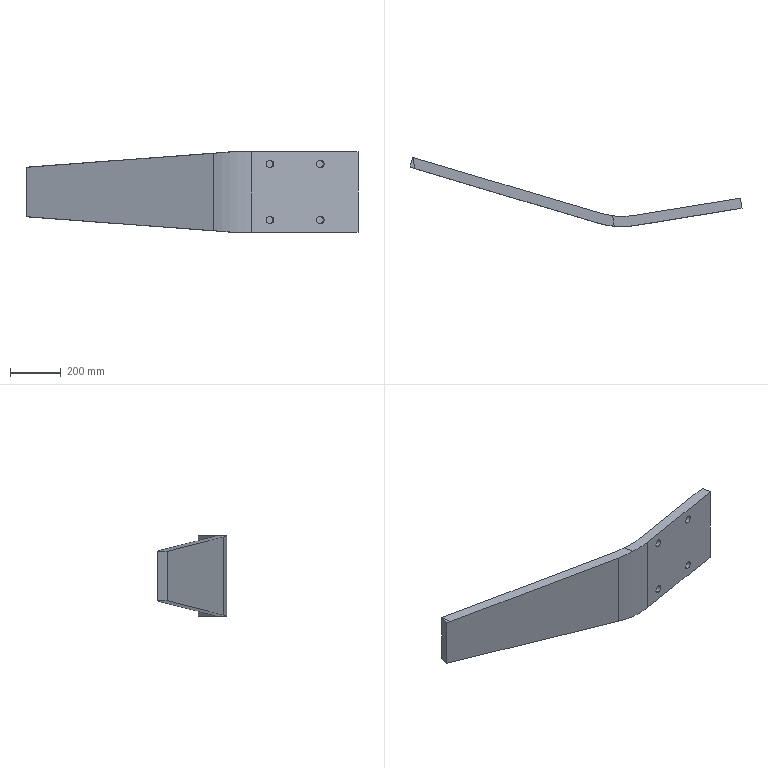Part | SolidWorks | features SplitBody 1 | 1 solid | 26 faces | box 1303 x 271.725 x 314 mm | volume 14705850 mm3 | plane 16 | cylinder 10 | commonest cylinder face diameters 30 x8 600 x1 680 x1
STEP:
#1=CARTESIAN_POINT('',(4308.613,120.712,-802.5));
#2=VERTEX_POINT('',#1);
#3=CARTESIAN_POINT('',(4308.613,120.712,-832.5));
#4=VERTEX_POINT('',#3);
#5=CARTESIAN_POINT('',(4308.613,120.712,-817.5));
#6=DIRECTION('',(0.1602,-0.9871,0.));
#7=DIRECTION('',(0.,0.,-1.));
#8=AXIS2_PLACEMENT_3D('',#5,#6,#7);
#9=CIRCLE('',#8,15.);
#10=EDGE_CURVE('',#2,#4,#9,.T.);
#11=ORIENTED_EDGE('',*,*,#10,.F.);
#12=CARTESIAN_POINT('',(4311.817,100.971,-802.5));
#13=VERTEX_POINT('',#12);
#14=CARTESIAN_POINT('',(4308.613,120.712,-802.5));
#15=DIRECTION('',(0.1602,-0.9871,0.));
#16=VECTOR('',#15,1000.);
#17=LINE('',#14,#16);
#18=EDGE_CURVE('',#2,#13,#17,.T.);
#19=ORIENTED_EDGE('',*,*,#18,.T.);
#20=CARTESIAN_POINT('',(4311.817,100.971,-832.5));
#21=VERTEX_POINT('',#20);
#22=CARTESIAN_POINT('',(4311.817,100.971,-817.5));
#23=DIRECTION('',(0.1602,-0.9871,0.));
#24=DIRECTION('',(0.,0.,-1.));
#25=AXIS2_PLACEMENT_3D('',#22,#23,#24);
#26=CIRCLE('',#25,15.);
#27=EDGE_CURVE('',#13,#21,#26,.T.);
#28=ORIENTED_EDGE('',*,*,#27,.T.);
#29=CARTESIAN_POINT('',(4308.613,120.712,-832.5));
#30=DIRECTION('',(0.1602,-0.9871,0.));
#31=VECTOR('',#30,1000.);
#32=LINE('',#29,#31);
#33=EDGE_CURVE('',#4,#21,#32,.T.);
#34=ORIENTED_EDGE('',*,*,#33,.F.);
#35=EDGE_LOOP('',(#11,#19,#28,#34));
#36=FACE_OUTER_BOUND('',#35,.T.);
#37=CARTESIAN_POINT('',(4308.613,120.712,-817.5));
#38=DIRECTION('',(0.1602,-0.9871,0.));
#39=DIRECTION('',(0.,0.,-1.));
#40=AXIS2_PLACEMENT_3D('',#37,#38,#39);
#41=CYLINDRICAL_SURFACE('',#40,15.);
#42=ADVANCED_FACE('',(#36),#41,.F.);
#43=CARTESIAN_POINT('',(4308.613,120.712,-1022.5));
#44=VERTEX_POINT('',#43);
#45=CARTESIAN_POINT('',(4308.613,120.712,-1052.5));
#46=VERTEX_POINT('',#45);
#47=CARTESIAN_POINT('',(4308.613,120.712,-1037.5));
#48=DIRECTION('',(0.1602,-0.9871,0.));
#49=DIRECTION('',(0.,0.,-1.));
#50=AXIS2_PLACEMENT_3D('',#47,#48,#49);
#51=CIRCLE('',#50,15.);
#52=EDGE_CURVE('',#44,#46,#51,.T.);
#53=ORIENTED_EDGE('',*,*,#52,.F.);
#54=CARTESIAN_POINT('',(4311.817,100.971,-1022.5));
#55=VERTEX_POINT('',#54);
#56=CARTESIAN_POINT('',(4308.613,120.712,-1022.5));
#57=DIRECTION('',(0.1602,-0.9871,0.));
#58=VECTOR('',#57,1000.);
#59=LINE('',#56,#58);
#60=EDGE_CURVE('',#44,#55,#59,.T.);
#61=ORIENTED_EDGE('',*,*,#60,.T.);
#62=CARTESIAN_POINT('',(4311.817,100.971,-1052.5));
#63=VERTEX_POINT('',#62);
#64=CARTESIAN_POINT('',(4311.817,100.971,-1037.5));
#65=DIRECTION('',(0.1602,-0.9871,0.));
#66=DIRECTION('',(0.,0.,-1.));
#67=AXIS2_PLACEMENT_3D('',#64,#65,#66);
#68=CIRCLE('',#67,15.);
#69=EDGE_CURVE('',#55,#63,#68,.T.);
#70=ORIENTED_EDGE('',*,*,#69,.T.);
#71=CARTESIAN_POINT('',(4308.613,120.712,-1052.5));
#72=DIRECTION('',(0.1602,-0.9871,0.));
#73=VECTOR('',#72,1000.);
#74=LINE('',#71,#73);
#75=EDGE_CURVE('',#46,#63,#74,.T.);
#76=ORIENTED_EDGE('',*,*,#75,.F.);
#77=EDGE_LOOP('',(#53,#61,#70,#76));
#78=FACE_OUTER_BOUND('',#77,.T.);
#79=CARTESIAN_POINT('',(4308.613,120.712,-1037.5));
#80=DIRECTION('',(0.1602,-0.9871,0.));
#81=DIRECTION('',(0.,0.,-1.));
#82=AXIS2_PLACEMENT_3D('',#79,#80,#81);
#83=CYLINDRICAL_SURFACE('',#82,15.);
#84=ADVANCED_FACE('',(#78),#83,.F.);
#85=CARTESIAN_POINT('',(4111.196,88.673,-802.5));
#86=VERTEX_POINT('',#85);
#87=CARTESIAN_POINT('',(4111.196,88.673,-832.5));
#88=VERTEX_POINT('',#87);
#89=CARTESIAN_POINT('',(4111.196,88.673,-817.5));
#90=DIRECTION('',(0.1602,-0.9871,0.));
#91=DIRECTION('',(0.,0.,-1.));
#92=AXIS2_PLACEMENT_3D('',#89,#90,#91);
#93=CIRCLE('',#92,15.);
#94=EDGE_CURVE('',#86,#88,#93,.T.);
#95=ORIENTED_EDGE('',*,*,#94,.F.);
#96=CARTESIAN_POINT('',(4114.4,68.931,-802.5));
#97=VERTEX_POINT('',#96);
#98=CARTESIAN_POINT('',(4111.196,88.673,-802.5));
#99=DIRECTION('',(0.1602,-0.9871,0.));
#100=VECTOR('',#99,1000.);
#101=LINE('',#98,#100);
#102=EDGE_CURVE('',#86,#97,#101,.T.);
#103=ORIENTED_EDGE('',*,*,#102,.T.);
#104=CARTESIAN_POINT('',(4114.4,68.931,-832.5));
#105=VERTEX_POINT('',#104);
#106=CARTESIAN_POINT('',(4114.4,68.931,-817.5));
#107=DIRECTION('',(0.1602,-0.9871,0.));
#108=DIRECTION('',(0.,0.,-1.));
#109=AXIS2_PLACEMENT_3D('',#106,#107,#108);
#110=CIRCLE('',#109,15.);
#111=EDGE_CURVE('',#97,#105,#110,.T.);
#112=ORIENTED_EDGE('',*,*,#111,.T.);
#113=CARTESIAN_POINT('',(4111.196,88.673,-832.5));
#114=DIRECTION('',(0.1602,-0.9871,0.));
#115=VECTOR('',#114,1000.);
#116=LINE('',#113,#115);
#117=EDGE_CURVE('',#88,#105,#116,.T.);
#118=ORIENTED_EDGE('',*,*,#117,.F.);
#119=EDGE_LOOP('',(#95,#103,#112,#118));
#120=FACE_OUTER_BOUND('',#119,.T.);
#121=CARTESIAN_POINT('',(4111.196,88.673,-817.5));
#122=DIRECTION('',(0.1602,-0.9871,0.));
#123=DIRECTION('',(0.,0.,-1.));
#124=AXIS2_PLACEMENT_3D('',#121,#122,#123);
#125=CYLINDRICAL_SURFACE('',#124,15.);
#126=ADVANCED_FACE('',(#120),#125,.F.);
#127=CARTESIAN_POINT('',(4111.196,88.673,-1022.5));
#128=VERTEX_POINT('',#127);
#129=CARTESIAN_POINT('',(4111.196,88.673,-1052.5));
#130=VERTEX_POINT('',#129);
#131=CARTESIAN_POINT('',(4111.196,88.673,-1037.5));
#132=DIRECTION('',(0.1602,-0.9871,0.));
#133=DIRECTION('',(0.,0.,-1.));
#134=AXIS2_PLACEMENT_3D('',#131,#132,#133);
#135=CIRCLE('',#134,15.);
#136=EDGE_CURVE('',#128,#130,#135,.T.);
#137=ORIENTED_EDGE('',*,*,#136,.F.);
#138=CARTESIAN_POINT('',(4114.4,68.931,-1022.5));
#139=VERTEX_POINT('',#138);
#140=CARTESIAN_POINT('',(4111.196,88.673,-1022.5));
#141=DIRECTION('',(0.1602,-0.9871,0.));
#142=VECTOR('',#141,1000.);
#143=LINE('',#140,#142);
#144=EDGE_CURVE('',#128,#139,#143,.T.);
#145=ORIENTED_EDGE('',*,*,#144,.T.);
#146=CARTESIAN_POINT('',(4114.4,68.931,-1052.5));
#147=VERTEX_POINT('',#146);
#148=CARTESIAN_POINT('',(4114.4,68.931,-1037.5));
#149=DIRECTION('',(0.1602,-0.9871,0.));
#150=DIRECTION('',(0.,0.,-1.));
#151=AXIS2_PLACEMENT_3D('',#148,#149,#150);
#152=CIRCLE('',#151,15.);
#153=EDGE_CURVE('',#139,#147,#152,.T.);
#154=ORIENTED_EDGE('',*,*,#153,.T.);
#155=CARTESIAN_POINT('',(4111.196,88.673,-1052.5));
#156=DIRECTION('',(0.1602,-0.9871,0.));
#157=VECTOR('',#156,1000.);
#158=LINE('',#155,#157);
#159=EDGE_CURVE('',#130,#147,#158,.T.);
#160=ORIENTED_EDGE('',*,*,#159,.F.);
#161=EDGE_LOOP('',(#137,#145,#154,#160));
#162=FACE_OUTER_BOUND('',#161,.T.);
#163=CARTESIAN_POINT('',(4111.196,88.673,-1037.5));
#164=DIRECTION('',(0.1602,-0.9871,0.));
#165=DIRECTION('',(0.,0.,-1.));
#166=AXIS2_PLACEMENT_3D('',#163,#164,#165);
#167=CYLINDRICAL_SURFACE('',#166,15.);
#168=ADVANCED_FACE('',(#162),#167,.F.);
#169=CARTESIAN_POINT('',(3168.64,324.729,-1025.5));
#170=VERTEX_POINT('',#169);
#171=CARTESIAN_POINT('',(3903.049,105.534,-1080.755));
#172=VERTEX_POINT('',#171);
#173=CARTESIAN_POINT('',(3168.64,324.729,-1025.5));
#174=DIRECTION('',(0.9557,-0.2853,-0.07191));
#175=VECTOR('',#174,1000.);
#176=LINE('',#173,#175);
#177=EDGE_CURVE('',#170,#172,#176,.T.);
#178=ORIENTED_EDGE('',*,*,#177,.F.);
#179=CARTESIAN_POINT('',(3168.64,324.729,-829.5));
#180=VERTEX_POINT('',#179);
#181=CARTESIAN_POINT('',(3168.64,324.729,-770.5));
#182=DIRECTION('',(0.,0.,-1.));
#183=VECTOR('',#182,1000.);
#184=LINE('',#181,#183);
#185=EDGE_CURVE('',#180,#170,#184,.T.);
#186=ORIENTED_EDGE('',*,*,#185,.F.);
#187=CARTESIAN_POINT('',(3903.049,105.534,-774.245));
#188=VERTEX_POINT('',#187);
#189=CARTESIAN_POINT('',(3903.049,105.534,-774.245));
#190=DIRECTION('',(-0.9557,0.2853,-0.07191));
#191=VECTOR('',#190,1000.);
#192=LINE('',#189,#191);
#193=EDGE_CURVE('',#188,#180,#192,.T.);
#194=ORIENTED_EDGE('',*,*,#193,.F.);
#195=CARTESIAN_POINT('',(3903.049,105.534,-770.5));
#196=DIRECTION('',(0.,0.,1.));
#197=VECTOR('',#196,1000.);
#198=LINE('',#195,#197);
#199=EDGE_CURVE('',#172,#188,#198,.T.);
#200=ORIENTED_EDGE('',*,*,#199,.F.);
#201=EDGE_LOOP('',(#178,#186,#194,#200));
#202=FACE_OUTER_BOUND('',#201,.T.);
#203=CARTESIAN_POINT('',(3168.64,324.729,-770.5));
#204=DIRECTION('',(-0.286,-0.9582,0.));
#205=DIRECTION('',(0.9582,-0.286,0.));
#206=AXIS2_PLACEMENT_3D('',#203,#204,#205);
#207=PLANE('',#206);
#208=ADVANCED_FACE('',(#202),#207,.F.);
#209=CARTESIAN_POINT('',(3952.085,95.265,-1084.5));
#210=VERTEX_POINT('',#209);
#211=CARTESIAN_POINT('',(3903.049,105.534,-1080.755));
#212=CARTESIAN_POINT('',(3919.089,100.747,-1081.961));
#213=CARTESIAN_POINT('',(3935.472,97.316,-1083.213));
#214=CARTESIAN_POINT('',(3952.085,95.265,-1084.5));
#215=(BOUNDED_CURVE()B_SPLINE_CURVE(3,(#211,#212,#213,#214),.UNSPECIFIED.,.F.,.T.)B_SPLINE_CURVE_WITH_KNOTS((4,4),(4.261,4.429),.UNSPECIFIED.)CURVE()GEOMETRIC_REPRESENTATION_ITEM()RATIONAL_B_SPLINE_CURVE((1.,0.9977,0.9977,1.))REPRESENTATION_ITEM(''));
#216=EDGE_CURVE('',#172,#210,#215,.T.);
#217=ORIENTED_EDGE('',*,*,#216,.F.);
#218=ORIENTED_EDGE('',*,*,#199,.T.);
#219=CARTESIAN_POINT('',(3952.085,95.265,-770.5));
#220=VERTEX_POINT('',#219);
#221=CARTESIAN_POINT('',(3952.085,95.265,-770.5));
#222=CARTESIAN_POINT('',(3935.472,97.316,-771.787));
#223=CARTESIAN_POINT('',(3919.089,100.747,-773.039));
#224=CARTESIAN_POINT('',(3903.049,105.534,-774.245));
#225=(BOUNDED_CURVE()B_SPLINE_CURVE(3,(#221,#222,#223,#224),.UNSPECIFIED.,.F.,.T.)B_SPLINE_CURVE_WITH_KNOTS((4,4),(4.996,5.163),.UNSPECIFIED.)CURVE()GEOMETRIC_REPRESENTATION_ITEM()RATIONAL_B_SPLINE_CURVE((1.,0.9977,0.9977,1.))REPRESENTATION_ITEM(''));
#226=EDGE_CURVE('',#220,#188,#225,.T.);
#227=ORIENTED_EDGE('',*,*,#226,.F.);
#228=CARTESIAN_POINT('',(4036.907,96.878,-770.5));
#229=VERTEX_POINT('',#228);
#230=CARTESIAN_POINT('',(3988.848,393.004,-770.5));
#231=DIRECTION('',(0.,0.,-1.));
#232=DIRECTION('',(-0.9871,-0.1602,0.));
#233=AXIS2_PLACEMENT_3D('',#230,#231,#232);
#234=CIRCLE('',#233,300.);
#235=EDGE_CURVE('',#229,#220,#234,.T.);
#236=ORIENTED_EDGE('',*,*,#235,.F.);
#237=CARTESIAN_POINT('',(4036.907,96.878,-1084.5));
#238=VERTEX_POINT('',#237);
#239=CARTESIAN_POINT('',(4036.907,96.878,-770.5));
#240=DIRECTION('',(0.,0.,1.));
#241=VECTOR('',#240,1000.);
#242=LINE('',#239,#241);
#243=EDGE_CURVE('',#238,#229,#242,.T.);
#244=ORIENTED_EDGE('',*,*,#243,.F.);
#245=CARTESIAN_POINT('',(3988.848,393.004,-1084.5));
#246=DIRECTION('',(0.,0.,1.));
#247=DIRECTION('',(-0.9871,-0.1602,0.));
#248=AXIS2_PLACEMENT_3D('',#245,#246,#247);
#249=CIRCLE('',#248,300.);
#250=EDGE_CURVE('',#210,#238,#249,.T.);
#251=ORIENTED_EDGE('',*,*,#250,.F.);
#252=EDGE_LOOP('',(#217,#218,#227,#236,#244,#251));
#253=FACE_OUTER_BOUND('',#252,.T.);
#254=CARTESIAN_POINT('',(3988.848,393.004,-770.5));
#255=DIRECTION('',(0.,0.,-1.));
#256=DIRECTION('',(-0.9871,-0.1602,0.));
#257=AXIS2_PLACEMENT_3D('',#254,#255,#256);
#258=CYLINDRICAL_SURFACE('',#257,300.);
#259=ADVANCED_FACE('',(#253),#258,.F.);
#260=ORIENTED_EDGE('',*,*,#177,.T.);
#261=ORIENTED_EDGE('',*,*,#216,.T.);
#262=CARTESIAN_POINT('',(3958.727,54.34,-1084.5));
#263=VERTEX_POINT('',#262);
#264=CARTESIAN_POINT('',(3960.415,43.941,-1084.5));
#265=DIRECTION('',(-0.1602,0.9871,0.));
#266=VECTOR('',#265,1000.);
#267=LINE('',#264,#266);
#268=EDGE_CURVE('',#263,#210,#267,.T.);
#269=ORIENTED_EDGE('',*,*,#268,.F.);
#270=CARTESIAN_POINT('',(3891.609,67.205,-1079.358));
#271=VERTEX_POINT('',#270);
#272=CARTESIAN_POINT('',(3891.609,67.205,-1079.358));
#273=CARTESIAN_POINT('',(3913.512,60.668,-1081.006));
#274=CARTESIAN_POINT('',(3935.96,56.365,-1082.726));
#275=CARTESIAN_POINT('',(3958.727,54.34,-1084.5));
#276=(BOUNDED_CURVE()B_SPLINE_CURVE(3,(#272,#273,#274,#275),.UNSPECIFIED.,.F.,.F.)B_SPLINE_CURVE_WITH_KNOTS((4,4),(4.261,4.463),.UNSPECIFIED.)CURVE()GEOMETRIC_REPRESENTATION_ITEM()RATIONAL_B_SPLINE_CURVE((1.,0.9966,0.9966,1.))REPRESENTATION_ITEM(''));
#277=EDGE_CURVE('',#271,#263,#276,.T.);
#278=ORIENTED_EDGE('',*,*,#277,.F.);
#279=CARTESIAN_POINT('',(3175.76,280.86,-1025.5));
#280=VERTEX_POINT('',#279);
#281=CARTESIAN_POINT('',(3175.76,280.86,-1025.5));
#282=DIRECTION('',(0.9557,-0.2853,-0.07191));
#283=VECTOR('',#282,1000.);
#284=LINE('',#281,#283);
#285=EDGE_CURVE('',#280,#271,#284,.T.);
#286=ORIENTED_EDGE('',*,*,#285,.F.);
#287=CARTESIAN_POINT('',(3233.36,-74.055,-1025.5));
#288=DIRECTION('',(0.1602,-0.9871,0.));
#289=VECTOR('',#288,1000.);
#290=LINE('',#287,#289);
#291=EDGE_CURVE('',#170,#280,#290,.T.);
#292=ORIENTED_EDGE('',*,*,#291,.F.);
#293=EDGE_LOOP('',(#260,#261,#269,#278,#286,#292));
#294=FACE_OUTER_BOUND('',#293,.T.);
#295=CARTESIAN_POINT('',(3960.415,43.941,-1084.5));
#296=DIRECTION('',(0.07881,0.01279,0.9968));
#297=DIRECTION('',(0.9839,0.1597,-0.07985));
#298=AXIS2_PLACEMENT_3D('',#295,#296,#297);
#299=PLANE('',#298);
#300=ADVANCED_FACE('',(#294),#299,.F.);
#301=CARTESIAN_POINT('',(3157.2,286.4,-1025.5));
#302=VERTEX_POINT('',#301);
#303=CARTESIAN_POINT('',(3168.64,324.729,-1025.5));
#304=DIRECTION('',(0.286,0.9582,0.));
#305=VECTOR('',#304,1000.);
#306=LINE('',#303,#305);
#307=EDGE_CURVE('',#302,#170,#306,.T.);
#308=ORIENTED_EDGE('',*,*,#307,.F.);
#309=CARTESIAN_POINT('',(3157.2,286.4,-829.5));
#310=VERTEX_POINT('',#309);
#311=CARTESIAN_POINT('',(3157.2,286.4,-770.5));
#312=DIRECTION('',(0.,0.,-1.));
#313=VECTOR('',#312,1000.);
#314=LINE('',#311,#313);
#315=EDGE_CURVE('',#310,#302,#314,.T.);
#316=ORIENTED_EDGE('',*,*,#315,.F.);
#317=CARTESIAN_POINT('',(3168.64,324.729,-829.5));
#318=DIRECTION('',(-0.286,-0.9582,0.));
#319=VECTOR('',#318,1000.);
#320=LINE('',#317,#319);
#321=EDGE_CURVE('',#180,#310,#320,.T.);
#322=ORIENTED_EDGE('',*,*,#321,.F.);
#323=ORIENTED_EDGE('',*,*,#185,.T.);
#324=EDGE_LOOP('',(#308,#316,#322,#323));
#325=FACE_OUTER_BOUND('',#324,.T.);
#326=CARTESIAN_POINT('',(3168.64,324.729,-770.5));
#327=DIRECTION('',(0.9582,-0.286,0.));
#328=DIRECTION('',(0.286,0.9582,0.));
#329=AXIS2_PLACEMENT_3D('',#326,#327,#328);
#330=PLANE('',#329);
#331=ADVANCED_FACE('',(#325),#330,.F.);
#332=CARTESIAN_POINT('',(3958.727,54.34,-770.5));
#333=VERTEX_POINT('',#332);
#334=CARTESIAN_POINT('',(3960.415,43.941,-770.5));
#335=DIRECTION('',(0.1602,-0.9871,0.));
#336=VECTOR('',#335,1000.);
#337=LINE('',#334,#336);
#338=EDGE_CURVE('',#220,#333,#337,.T.);
#339=ORIENTED_EDGE('',*,*,#338,.F.);
#340=ORIENTED_EDGE('',*,*,#226,.T.);
#341=ORIENTED_EDGE('',*,*,#193,.T.);
#342=CARTESIAN_POINT('',(3175.76,280.86,-829.5));
#343=VERTEX_POINT('',#342);
#344=CARTESIAN_POINT('',(3233.36,-74.055,-829.5));
#345=DIRECTION('',(-0.1602,0.9871,0.));
#346=VECTOR('',#345,1000.);
#347=LINE('',#344,#346);
#348=EDGE_CURVE('',#343,#180,#347,.T.);
#349=ORIENTED_EDGE('',*,*,#348,.F.);
#350=CARTESIAN_POINT('',(3891.609,67.205,-775.642));
#351=VERTEX_POINT('',#350);
#352=CARTESIAN_POINT('',(3891.609,67.205,-775.642));
#353=DIRECTION('',(-0.9557,0.2853,-0.07191));
#354=VECTOR('',#353,1000.);
#355=LINE('',#352,#354);
#356=EDGE_CURVE('',#351,#343,#355,.T.);
#357=ORIENTED_EDGE('',*,*,#356,.F.);
#358=CARTESIAN_POINT('',(3958.727,54.34,-770.5));
#359=CARTESIAN_POINT('',(3935.96,56.365,-772.274));
#360=CARTESIAN_POINT('',(3913.512,60.668,-773.994));
#361=CARTESIAN_POINT('',(3891.609,67.205,-775.642));
#362=(BOUNDED_CURVE()B_SPLINE_CURVE(3,(#358,#359,#360,#361),.UNSPECIFIED.,.F.,.T.)B_SPLINE_CURVE_WITH_KNOTS((4,4),(4.962,5.163),.UNSPECIFIED.)CURVE()GEOMETRIC_REPRESENTATION_ITEM()RATIONAL_B_SPLINE_CURVE((1.,0.9966,0.9966,1.))REPRESENTATION_ITEM(''));
#363=EDGE_CURVE('',#333,#351,#362,.T.);
#364=ORIENTED_EDGE('',*,*,#363,.F.);
#365=EDGE_LOOP('',(#339,#340,#341,#349,#357,#364));
#366=FACE_OUTER_BOUND('',#365,.T.);
#367=CARTESIAN_POINT('',(3960.415,43.941,-770.5));
#368=DIRECTION('',(0.07881,0.01279,-0.9968));
#369=DIRECTION('',(-0.9839,-0.1597,-0.07985));
#370=AXIS2_PLACEMENT_3D('',#367,#368,#369);
#371=PLANE('',#370);
#372=ADVANCED_FACE('',(#366),#371,.F.);
#373=CARTESIAN_POINT('',(4459.88,125.,-1084.5));
#374=VERTEX_POINT('',#373);
#375=CARTESIAN_POINT('',(4043.315,57.395,-1084.5));
#376=VERTEX_POINT('',#375);
#377=CARTESIAN_POINT('',(4043.315,57.395,-1084.5));
#378=DIRECTION('',(-0.9871,-0.1602,0.));
#379=VECTOR('',#378,1000.);
#380=LINE('',#377,#379);
#381=EDGE_CURVE('',#374,#376,#380,.T.);
#382=ORIENTED_EDGE('',*,*,#381,.T.);
#383=CARTESIAN_POINT('',(3988.848,393.004,-1084.5));
#384=DIRECTION('',(0.,0.,-1.));
#385=DIRECTION('',(-0.9871,-0.1602,0.));
#386=AXIS2_PLACEMENT_3D('',#383,#384,#385);
#387=CIRCLE('',#386,340.);
#388=EDGE_CURVE('',#376,#263,#387,.T.);
#389=ORIENTED_EDGE('',*,*,#388,.T.);
#390=ORIENTED_EDGE('',*,*,#268,.T.);
#391=ORIENTED_EDGE('',*,*,#250,.T.);
#392=CARTESIAN_POINT('',(4453.472,164.483,-1084.5));
#393=VERTEX_POINT('',#392);
#394=CARTESIAN_POINT('',(4036.907,96.878,-1084.5));
#395=DIRECTION('',(0.9871,0.1602,0.));
#396=VECTOR('',#395,1000.);
#397=LINE('',#394,#396);
#398=EDGE_CURVE('',#238,#393,#397,.T.);
#399=ORIENTED_EDGE('',*,*,#398,.T.);
#400=CARTESIAN_POINT('',(4405.413,460.609,-1084.5));
#401=DIRECTION('',(0.1602,-0.9871,0.));
#402=VECTOR('',#401,1000.);
#403=LINE('',#400,#402);
#404=EDGE_CURVE('',#393,#374,#403,.T.);
#405=ORIENTED_EDGE('',*,*,#404,.T.);
#406=EDGE_LOOP('',(#382,#389,#390,#391,#399,#405));
#407=FACE_OUTER_BOUND('',#406,.T.);
#408=CARTESIAN_POINT('',(3988.848,393.004,-1084.5));
#409=DIRECTION('',(0.,0.,-1.));
#410=DIRECTION('',(-0.9871,-0.1602,0.));
#411=AXIS2_PLACEMENT_3D('',#408,#409,#410);
#412=PLANE('',#411);
#413=ADVANCED_FACE('',(#407),#412,.T.);
#414=ORIENTED_EDGE('',*,*,#338,.T.);
#415=CARTESIAN_POINT('',(4043.315,57.395,-770.5));
#416=VERTEX_POINT('',#415);
#417=CARTESIAN_POINT('',(3988.848,393.004,-770.5));
#418=DIRECTION('',(0.,0.,-1.));
#419=DIRECTION('',(-0.9871,-0.1602,0.));
#420=AXIS2_PLACEMENT_3D('',#417,#418,#419);
#421=CIRCLE('',#420,340.);
#422=EDGE_CURVE('',#416,#333,#421,.T.);
#423=ORIENTED_EDGE('',*,*,#422,.F.);
#424=CARTESIAN_POINT('',(4459.88,125.,-770.5));
#425=VERTEX_POINT('',#424);
#426=CARTESIAN_POINT('',(4043.315,57.395,-770.5));
#427=DIRECTION('',(-0.9871,-0.1602,0.));
#428=VECTOR('',#427,1000.);
#429=LINE('',#426,#428);
#430=EDGE_CURVE('',#425,#416,#429,.T.);
#431=ORIENTED_EDGE('',*,*,#430,.F.);
#432=CARTESIAN_POINT('',(4453.472,164.483,-770.5));
#433=VERTEX_POINT('',#432);
#434=CARTESIAN_POINT('',(4405.413,460.609,-770.5));
#435=DIRECTION('',(0.1602,-0.9871,0.));
#436=VECTOR('',#435,1000.);
#437=LINE('',#434,#436);
#438=EDGE_CURVE('',#433,#425,#437,.T.);
#439=ORIENTED_EDGE('',*,*,#438,.F.);
#440=CARTESIAN_POINT('',(4036.907,96.878,-770.5));
#441=DIRECTION('',(0.9871,0.1602,0.));
#442=VECTOR('',#441,1000.);
#443=LINE('',#440,#442);
#444=EDGE_CURVE('',#229,#433,#443,.T.);
#445=ORIENTED_EDGE('',*,*,#444,.F.);
#446=ORIENTED_EDGE('',*,*,#235,.T.);
#447=EDGE_LOOP('',(#414,#423,#431,#439,#445,#446));
#448=FACE_OUTER_BOUND('',#447,.T.);
#449=CARTESIAN_POINT('',(3988.848,393.004,-770.5));
#450=DIRECTION('',(0.,0.,-1.));
#451=DIRECTION('',(-0.9871,-0.1602,0.));
#452=AXIS2_PLACEMENT_3D('',#449,#450,#451);
#453=PLANE('',#452);
#454=ADVANCED_FACE('',(#448),#453,.F.);
#455=ORIENTED_EDGE('',*,*,#243,.T.);
#456=ORIENTED_EDGE('',*,*,#444,.T.);
#457=CARTESIAN_POINT('',(4453.472,164.483,-770.5));
#458=DIRECTION('',(0.,0.,1.));
#459=VECTOR('',#458,1000.);
#460=LINE('',#457,#459);
#461=EDGE_CURVE('',#393,#433,#460,.T.);
#462=ORIENTED_EDGE('',*,*,#461,.F.);
#463=ORIENTED_EDGE('',*,*,#398,.F.);
#464=EDGE_LOOP('',(#455,#456,#462,#463));
#465=FACE_OUTER_BOUND('',#464,.T.);
#466=CARTESIAN_POINT('',(4036.907,96.878,-770.5));
#467=DIRECTION('',(0.1602,-0.9871,0.));
#468=DIRECTION('',(0.9871,0.1602,0.));
#469=AXIS2_PLACEMENT_3D('',#466,#467,#468);
#470=PLANE('',#469);
#471=ADVANCED_FACE('',(#465),#470,.F.);
#472=CARTESIAN_POINT('',(3157.2,286.4,-1025.5));
#473=DIRECTION('',(0.9582,-0.286,0.));
#474=VECTOR('',#473,1000.);
#475=LINE('',#472,#474);
#476=EDGE_CURVE('',#302,#280,#475,.T.);
#477=ORIENTED_EDGE('',*,*,#476,.F.);
#478=ORIENTED_EDGE('',*,*,#307,.T.);
#479=ORIENTED_EDGE('',*,*,#291,.T.);
#480=EDGE_LOOP('',(#477,#478,#479));
#481=FACE_OUTER_BOUND('',#480,.T.);
#482=CARTESIAN_POINT('',(3233.36,-74.055,-1025.5));
#483=DIRECTION('',(0.,0.,1.));
#484=DIRECTION('',(0.9871,0.1602,0.));
#485=AXIS2_PLACEMENT_3D('',#482,#483,#484);
#486=PLANE('',#485);
#487=ADVANCED_FACE('',(#481),#486,.F.);
#488=ORIENTED_EDGE('',*,*,#422,.T.);
#489=ORIENTED_EDGE('',*,*,#363,.T.);
#490=CARTESIAN_POINT('',(3891.609,67.205,-770.5));
#491=DIRECTION('',(0.,0.,-1.));
#492=VECTOR('',#491,1000.);
#493=LINE('',#490,#492);
#494=EDGE_CURVE('',#351,#271,#493,.T.);
#495=ORIENTED_EDGE('',*,*,#494,.T.);
#496=ORIENTED_EDGE('',*,*,#277,.T.);
#497=ORIENTED_EDGE('',*,*,#388,.F.);
#498=CARTESIAN_POINT('',(4043.315,57.395,-770.5));
#499=DIRECTION('',(0.,0.,1.));
#500=VECTOR('',#499,1000.);
#501=LINE('',#498,#500);
#502=EDGE_CURVE('',#376,#416,#501,.T.);
#503=ORIENTED_EDGE('',*,*,#502,.T.);
#504=EDGE_LOOP('',(#488,#489,#495,#496,#497,#503));
#505=FACE_OUTER_BOUND('',#504,.T.);
#506=CARTESIAN_POINT('',(3988.848,393.004,-770.5));
#507=DIRECTION('',(0.,0.,-1.));
#508=DIRECTION('',(-0.9871,-0.1602,0.));
#509=AXIS2_PLACEMENT_3D('',#506,#507,#508);
#510=CYLINDRICAL_SURFACE('',#509,340.);
#511=ADVANCED_FACE('',(#505),#510,.T.);
#512=ORIENTED_EDGE('',*,*,#285,.T.);
#513=ORIENTED_EDGE('',*,*,#494,.F.);
#514=ORIENTED_EDGE('',*,*,#356,.T.);
#515=CARTESIAN_POINT('',(3157.2,286.4,-829.5));
#516=DIRECTION('',(0.9582,-0.286,0.));
#517=VECTOR('',#516,1000.);
#518=LINE('',#515,#517);
#519=EDGE_CURVE('',#310,#343,#518,.T.);
#520=ORIENTED_EDGE('',*,*,#519,.F.);
#521=ORIENTED_EDGE('',*,*,#315,.T.);
#522=ORIENTED_EDGE('',*,*,#476,.T.);
#523=EDGE_LOOP('',(#512,#513,#514,#520,#521,#522));
#524=FACE_OUTER_BOUND('',#523,.T.);
#525=CARTESIAN_POINT('',(3157.2,286.4,-770.5));
#526=DIRECTION('',(0.286,0.9582,0.));
#527=DIRECTION('',(-0.9582,0.286,0.));
#528=AXIS2_PLACEMENT_3D('',#525,#526,#527);
#529=PLANE('',#528);
#530=ADVANCED_FACE('',(#524),#529,.F.);
#531=ORIENTED_EDGE('',*,*,#348,.T.);
#532=ORIENTED_EDGE('',*,*,#321,.T.);
#533=ORIENTED_EDGE('',*,*,#519,.T.);
#534=EDGE_LOOP('',(#531,#532,#533));
#535=FACE_OUTER_BOUND('',#534,.T.);
#536=CARTESIAN_POINT('',(3233.36,-74.055,-829.5));
#537=DIRECTION('',(0.,0.,-1.));
#538=DIRECTION('',(-0.9871,-0.1602,0.));
#539=AXIS2_PLACEMENT_3D('',#536,#537,#538);
#540=PLANE('',#539);
#541=ADVANCED_FACE('',(#535),#540,.F.);
#542=CARTESIAN_POINT('',(4459.88,125.,-770.5));
#543=DIRECTION('',(0.,0.,-1.));
#544=VECTOR('',#543,1000.);
#545=LINE('',#542,#544);
#546=EDGE_CURVE('',#425,#374,#545,.T.);
#547=ORIENTED_EDGE('',*,*,#546,.F.);
#548=ORIENTED_EDGE('',*,*,#430,.T.);
#549=ORIENTED_EDGE('',*,*,#502,.F.);
#550=ORIENTED_EDGE('',*,*,#381,.F.);
#551=EDGE_LOOP('',(#547,#548,#549,#550));
#552=FACE_OUTER_BOUND('',#551,.T.);
#553=CARTESIAN_POINT('',(4311.817,100.971,-817.5));
#554=DIRECTION('',(0.1602,-0.9871,0.));
#555=DIRECTION('',(0.,0.,-1.));
#556=AXIS2_PLACEMENT_3D('',#553,#554,#555);
#557=CIRCLE('',#556,15.);
#558=EDGE_CURVE('',#21,#13,#557,.T.);
#559=ORIENTED_EDGE('',*,*,#558,.F.);
#560=ORIENTED_EDGE('',*,*,#27,.F.);
#561=EDGE_LOOP('',(#559,#560));
#562=FACE_BOUND('',#561,.T.);
#563=CARTESIAN_POINT('',(4311.817,100.971,-1037.5));
#564=DIRECTION('',(0.1602,-0.9871,0.));
#565=DIRECTION('',(0.,0.,-1.));
#566=AXIS2_PLACEMENT_3D('',#563,#564,#565);
#567=CIRCLE('',#566,15.);
#568=EDGE_CURVE('',#63,#55,#567,.T.);
#569=ORIENTED_EDGE('',*,*,#568,.F.);
#570=ORIENTED_EDGE('',*,*,#69,.F.);
#571=EDGE_LOOP('',(#569,#570));
#572=FACE_BOUND('',#571,.T.);
#573=CARTESIAN_POINT('',(4114.4,68.931,-817.5));
#574=DIRECTION('',(0.1602,-0.9871,0.));
#575=DIRECTION('',(0.,0.,-1.));
#576=AXIS2_PLACEMENT_3D('',#573,#574,#575);
#577=CIRCLE('',#576,15.);
#578=EDGE_CURVE('',#105,#97,#577,.T.);
#579=ORIENTED_EDGE('',*,*,#578,.F.);
#580=ORIENTED_EDGE('',*,*,#111,.F.);
#581=EDGE_LOOP('',(#579,#580));
#582=FACE_BOUND('',#581,.T.);
#583=CARTESIAN_POINT('',(4114.4,68.931,-1037.5));
#584=DIRECTION('',(0.1602,-0.9871,0.));
#585=DIRECTION('',(0.,0.,-1.));
#586=AXIS2_PLACEMENT_3D('',#583,#584,#585);
#587=CIRCLE('',#586,15.);
#588=EDGE_CURVE('',#147,#139,#587,.T.);
#589=ORIENTED_EDGE('',*,*,#588,.F.);
#590=ORIENTED_EDGE('',*,*,#153,.F.);
#591=EDGE_LOOP('',(#589,#590));
#592=FACE_BOUND('',#591,.T.);
#593=CARTESIAN_POINT('',(4043.315,57.395,-770.5));
#594=DIRECTION('',(-0.1602,0.9871,0.));
#595=DIRECTION('',(0.,0.,1.));
#596=AXIS2_PLACEMENT_3D('',#593,#594,#595);
#597=PLANE('',#596);
#598=ADVANCED_FACE('',(#552,#562,#572,#582,#592),#597,.F.);
#599=ORIENTED_EDGE('',*,*,#461,.T.);
#600=ORIENTED_EDGE('',*,*,#438,.T.);
#601=ORIENTED_EDGE('',*,*,#546,.T.);
#602=ORIENTED_EDGE('',*,*,#404,.F.);
#603=EDGE_LOOP('',(#599,#600,#601,#602));
#604=FACE_OUTER_BOUND('',#603,.T.);
#605=CARTESIAN_POINT('',(4453.472,164.483,-770.5));
#606=DIRECTION('',(-0.9871,-0.1602,0.));
#607=DIRECTION('',(0.,0.,1.));
#608=AXIS2_PLACEMENT_3D('',#605,#606,#607);
#609=PLANE('',#608);
#610=ADVANCED_FACE('',(#604),#609,.F.);
#611=ORIENTED_EDGE('',*,*,#18,.F.);
#612=CARTESIAN_POINT('',(4308.613,120.712,-817.5));
#613=DIRECTION('',(0.1602,-0.9871,0.));
#614=DIRECTION('',(0.,0.,-1.));
#615=AXIS2_PLACEMENT_3D('',#612,#613,#614);
#616=CIRCLE('',#615,15.);
#617=EDGE_CURVE('',#4,#2,#616,.T.);
#618=ORIENTED_EDGE('',*,*,#617,.F.);
#619=ORIENTED_EDGE('',*,*,#33,.T.);
#620=ORIENTED_EDGE('',*,*,#558,.T.);
#621=EDGE_LOOP('',(#611,#618,#619,#620));
#622=FACE_OUTER_BOUND('',#621,.T.);
#623=CARTESIAN_POINT('',(4308.613,120.712,-817.5));
#624=DIRECTION('',(0.1602,-0.9871,0.));
#625=DIRECTION('',(0.,0.,-1.));
#626=AXIS2_PLACEMENT_3D('',#623,#624,#625);
#627=CYLINDRICAL_SURFACE('',#626,15.);
#628=ADVANCED_FACE('',(#622),#627,.F.);
#629=ORIENTED_EDGE('',*,*,#60,.F.);
#630=CARTESIAN_POINT('',(4308.613,120.712,-1037.5));
#631=DIRECTION('',(0.1602,-0.9871,0.));
#632=DIRECTION('',(0.,0.,-1.));
#633=AXIS2_PLACEMENT_3D('',#630,#631,#632);
#634=CIRCLE('',#633,15.);
#635=EDGE_CURVE('',#46,#44,#634,.T.);
#636=ORIENTED_EDGE('',*,*,#635,.F.);
#637=ORIENTED_EDGE('',*,*,#75,.T.);
#638=ORIENTED_EDGE('',*,*,#568,.T.);
#639=EDGE_LOOP('',(#629,#636,#637,#638));
#640=FACE_OUTER_BOUND('',#639,.T.);
#641=CARTESIAN_POINT('',(4308.613,120.712,-1037.5));
#642=DIRECTION('',(0.1602,-0.9871,0.));
#643=DIRECTION('',(0.,0.,-1.));
#644=AXIS2_PLACEMENT_3D('',#641,#642,#643);
#645=CYLINDRICAL_SURFACE('',#644,15.);
#646=ADVANCED_FACE('',(#640),#645,.F.);
#647=ORIENTED_EDGE('',*,*,#102,.F.);
#648=CARTESIAN_POINT('',(4111.196,88.673,-817.5));
#649=DIRECTION('',(0.1602,-0.9871,0.));
#650=DIRECTION('',(0.,0.,-1.));
#651=AXIS2_PLACEMENT_3D('',#648,#649,#650);
#652=CIRCLE('',#651,15.);
#653=EDGE_CURVE('',#88,#86,#652,.T.);
#654=ORIENTED_EDGE('',*,*,#653,.F.);
#655=ORIENTED_EDGE('',*,*,#117,.T.);
#656=ORIENTED_EDGE('',*,*,#578,.T.);
#657=EDGE_LOOP('',(#647,#654,#655,#656));
#658=FACE_OUTER_BOUND('',#657,.T.);
#659=CARTESIAN_POINT('',(4111.196,88.673,-817.5));
#660=DIRECTION('',(0.1602,-0.9871,0.));
#661=DIRECTION('',(0.,0.,-1.));
#662=AXIS2_PLACEMENT_3D('',#659,#660,#661);
#663=CYLINDRICAL_SURFACE('',#662,15.);
#664=ADVANCED_FACE('',(#658),#663,.F.);
#665=ORIENTED_EDGE('',*,*,#144,.F.);
#666=CARTESIAN_POINT('',(4111.196,88.673,-1037.5));
#667=DIRECTION('',(0.1602,-0.9871,0.));
#668=DIRECTION('',(0.,0.,-1.));
#669=AXIS2_PLACEMENT_3D('',#666,#667,#668);
#670=CIRCLE('',#669,15.);
#671=EDGE_CURVE('',#130,#128,#670,.T.);
#672=ORIENTED_EDGE('',*,*,#671,.F.);
#673=ORIENTED_EDGE('',*,*,#159,.T.);
#674=ORIENTED_EDGE('',*,*,#588,.T.);
#675=EDGE_LOOP('',(#665,#672,#673,#674));
#676=FACE_OUTER_BOUND('',#675,.T.);
#677=CARTESIAN_POINT('',(4111.196,88.673,-1037.5));
#678=DIRECTION('',(0.1602,-0.9871,0.));
#679=DIRECTION('',(0.,0.,-1.));
#680=AXIS2_PLACEMENT_3D('',#677,#678,#679);
#681=CYLINDRICAL_SURFACE('',#680,15.);
#682=ADVANCED_FACE('',(#676),#681,.F.);
#683=ORIENTED_EDGE('',*,*,#617,.T.);
#684=ORIENTED_EDGE('',*,*,#10,.T.);
#685=EDGE_LOOP('',(#683,#684));
#686=FACE_OUTER_BOUND('',#685,.T.);
#687=CARTESIAN_POINT('',(4308.613,120.712,-817.5));
#688=DIRECTION('',(0.1602,-0.9871,0.));
#689=DIRECTION('',(0.,0.,-1.));
#690=AXIS2_PLACEMENT_3D('',#687,#688,#689);
#691=PLANE('',#690);
#692=ADVANCED_FACE('',(#686),#691,.T.);
#693=ORIENTED_EDGE('',*,*,#635,.T.);
#694=ORIENTED_EDGE('',*,*,#52,.T.);
#695=EDGE_LOOP('',(#693,#694));
#696=FACE_OUTER_BOUND('',#695,.T.);
#697=CARTESIAN_POINT('',(4308.613,120.712,-1037.5));
#698=DIRECTION('',(0.1602,-0.9871,0.));
#699=DIRECTION('',(0.,0.,-1.));
#700=AXIS2_PLACEMENT_3D('',#697,#698,#699);
#701=PLANE('',#700);
#702=ADVANCED_FACE('',(#696),#701,.T.);
#703=ORIENTED_EDGE('',*,*,#653,.T.);
#704=ORIENTED_EDGE('',*,*,#94,.T.);
#705=EDGE_LOOP('',(#703,#704));
#706=FACE_OUTER_BOUND('',#705,.T.);
#707=CARTESIAN_POINT('',(4111.196,88.673,-817.5));
#708=DIRECTION('',(0.1602,-0.9871,0.));
#709=DIRECTION('',(0.,0.,-1.));
#710=AXIS2_PLACEMENT_3D('',#707,#708,#709);
#711=PLANE('',#710);
#712=ADVANCED_FACE('',(#706),#711,.T.);
#713=ORIENTED_EDGE('',*,*,#671,.T.);
#714=ORIENTED_EDGE('',*,*,#136,.T.);
#715=EDGE_LOOP('',(#713,#714));
#716=FACE_OUTER_BOUND('',#715,.T.);
#717=CARTESIAN_POINT('',(4111.196,88.673,-1037.5));
#718=DIRECTION('',(0.1602,-0.9871,0.));
#719=DIRECTION('',(0.,0.,-1.));
#720=AXIS2_PLACEMENT_3D('',#717,#718,#719);
#721=PLANE('',#720);
#722=ADVANCED_FACE('',(#716),#721,.T.);
#723=CLOSED_SHELL('',(#42,#84,#126,#168,#208,#259,#300,#331,#372,#413,#454,#471,#487,#511,#530,#541,#598,#610,#628,#646,#664,#682,#692,#702,#712,#722));
#724=MANIFOLD_SOLID_BREP('',#723);
#725=CARTESIAN_POINT('',(0.,0.,0.));
#726=DIRECTION('',(0.,0.,1.));
#727=DIRECTION('',(1.,0.,0.));
#728=AXIS2_PLACEMENT_3D('',#725,#726,#727);
#729=(LENGTH_UNIT()NAMED_UNIT(*)SI_UNIT(.MILLI.,.METRE.));
#730=UNCERTAINTY_MEASURE_WITH_UNIT(LENGTH_MEASURE(0.00001),#729,'','');
#731=(NAMED_UNIT(*)PLANE_ANGLE_UNIT()SI_UNIT($,.RADIAN.));
#732=(NAMED_UNIT(*)SI_UNIT($,.STERADIAN.)SOLID_ANGLE_UNIT());
#733=(GEOMETRIC_REPRESENTATION_CONTEXT(3)GLOBAL_UNCERTAINTY_ASSIGNED_CONTEXT((#730))GLOBAL_UNIT_ASSIGNED_CONTEXT((#729,#731,#732))REPRESENTATION_CONTEXT('',''));
#734=ADVANCED_BREP_SHAPE_REPRESENTATION('',(#724,#728),#733);